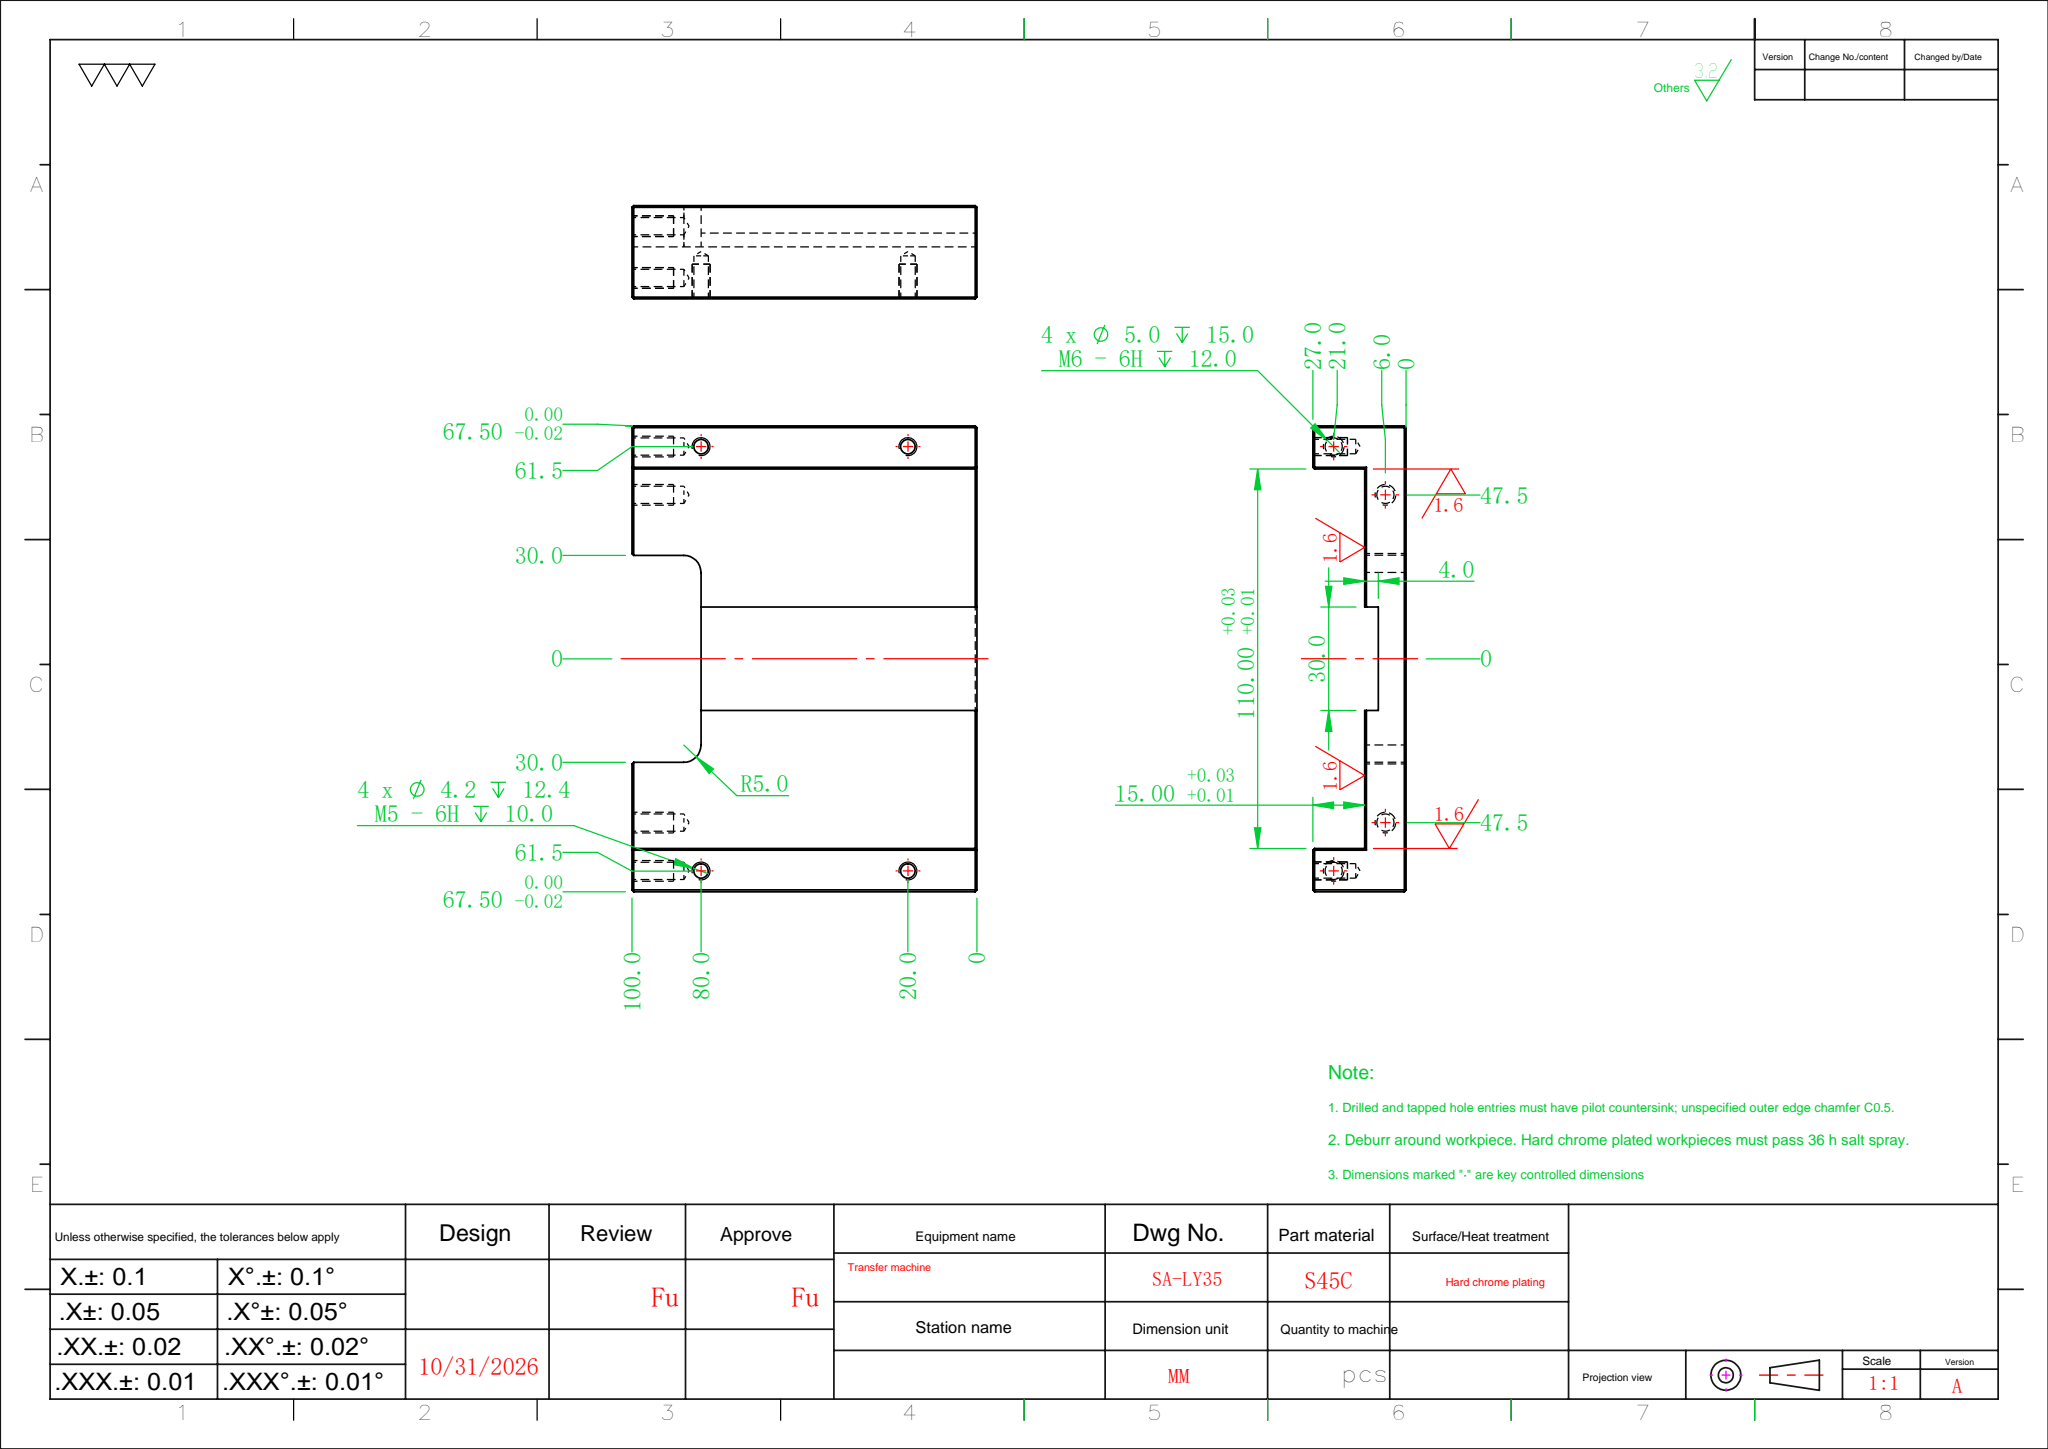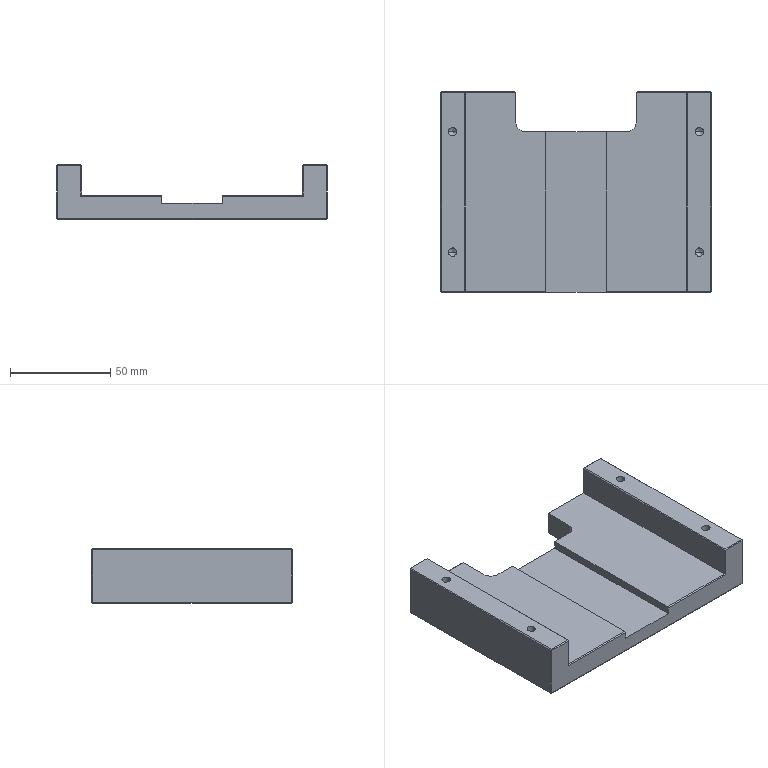Part | SolidWorks | features HoleWzd 2, ICE 2, Chamfer 1, Cut 1, Extrusion 1, Fillet 1 | 1 solid | 91 faces | box 135 x 100 x 27 mm | volume 173554 mm3 | plane 57 | cylinder 18 | cone 16 | commonest cylinder face diameters 4.2 x8 5 x8 10 x2